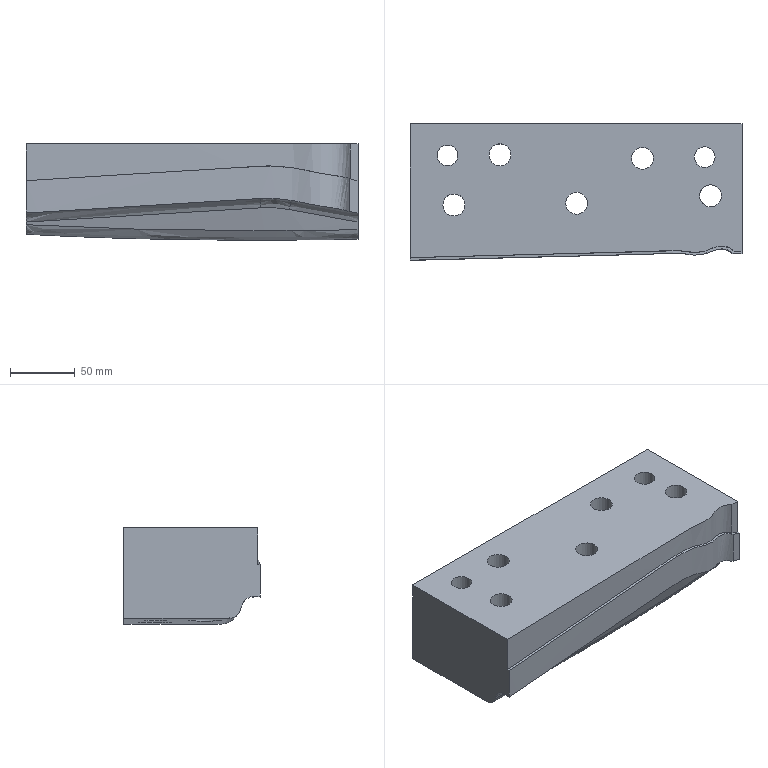Part | NX | features solid 2 | 1 solid | 39 faces | box 257 x 105.627 x 74.563 mm | volume 1649515 mm3 | cylinder 14 | spline 13 | plane 12 | commonest cylinder face diameters 17 x7 25 x5 16 x2